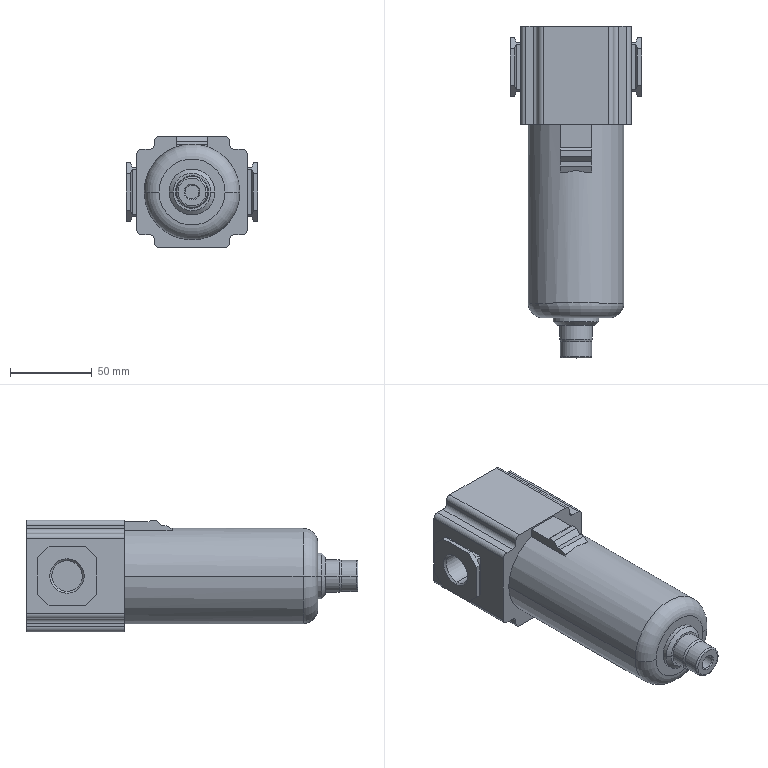Part | SolidWorks | features BaseBody 1 | 1 solid | 104 faces | box 80 x 202.5 x 68 mm | volume 579205 mm3 | plane 64 | cylinder 26 | cone 10 | torus 4 | commonest cylinder face diameters 6 x12 18.631 x4 8.566 x2 19 x2 20 x2 28 x2